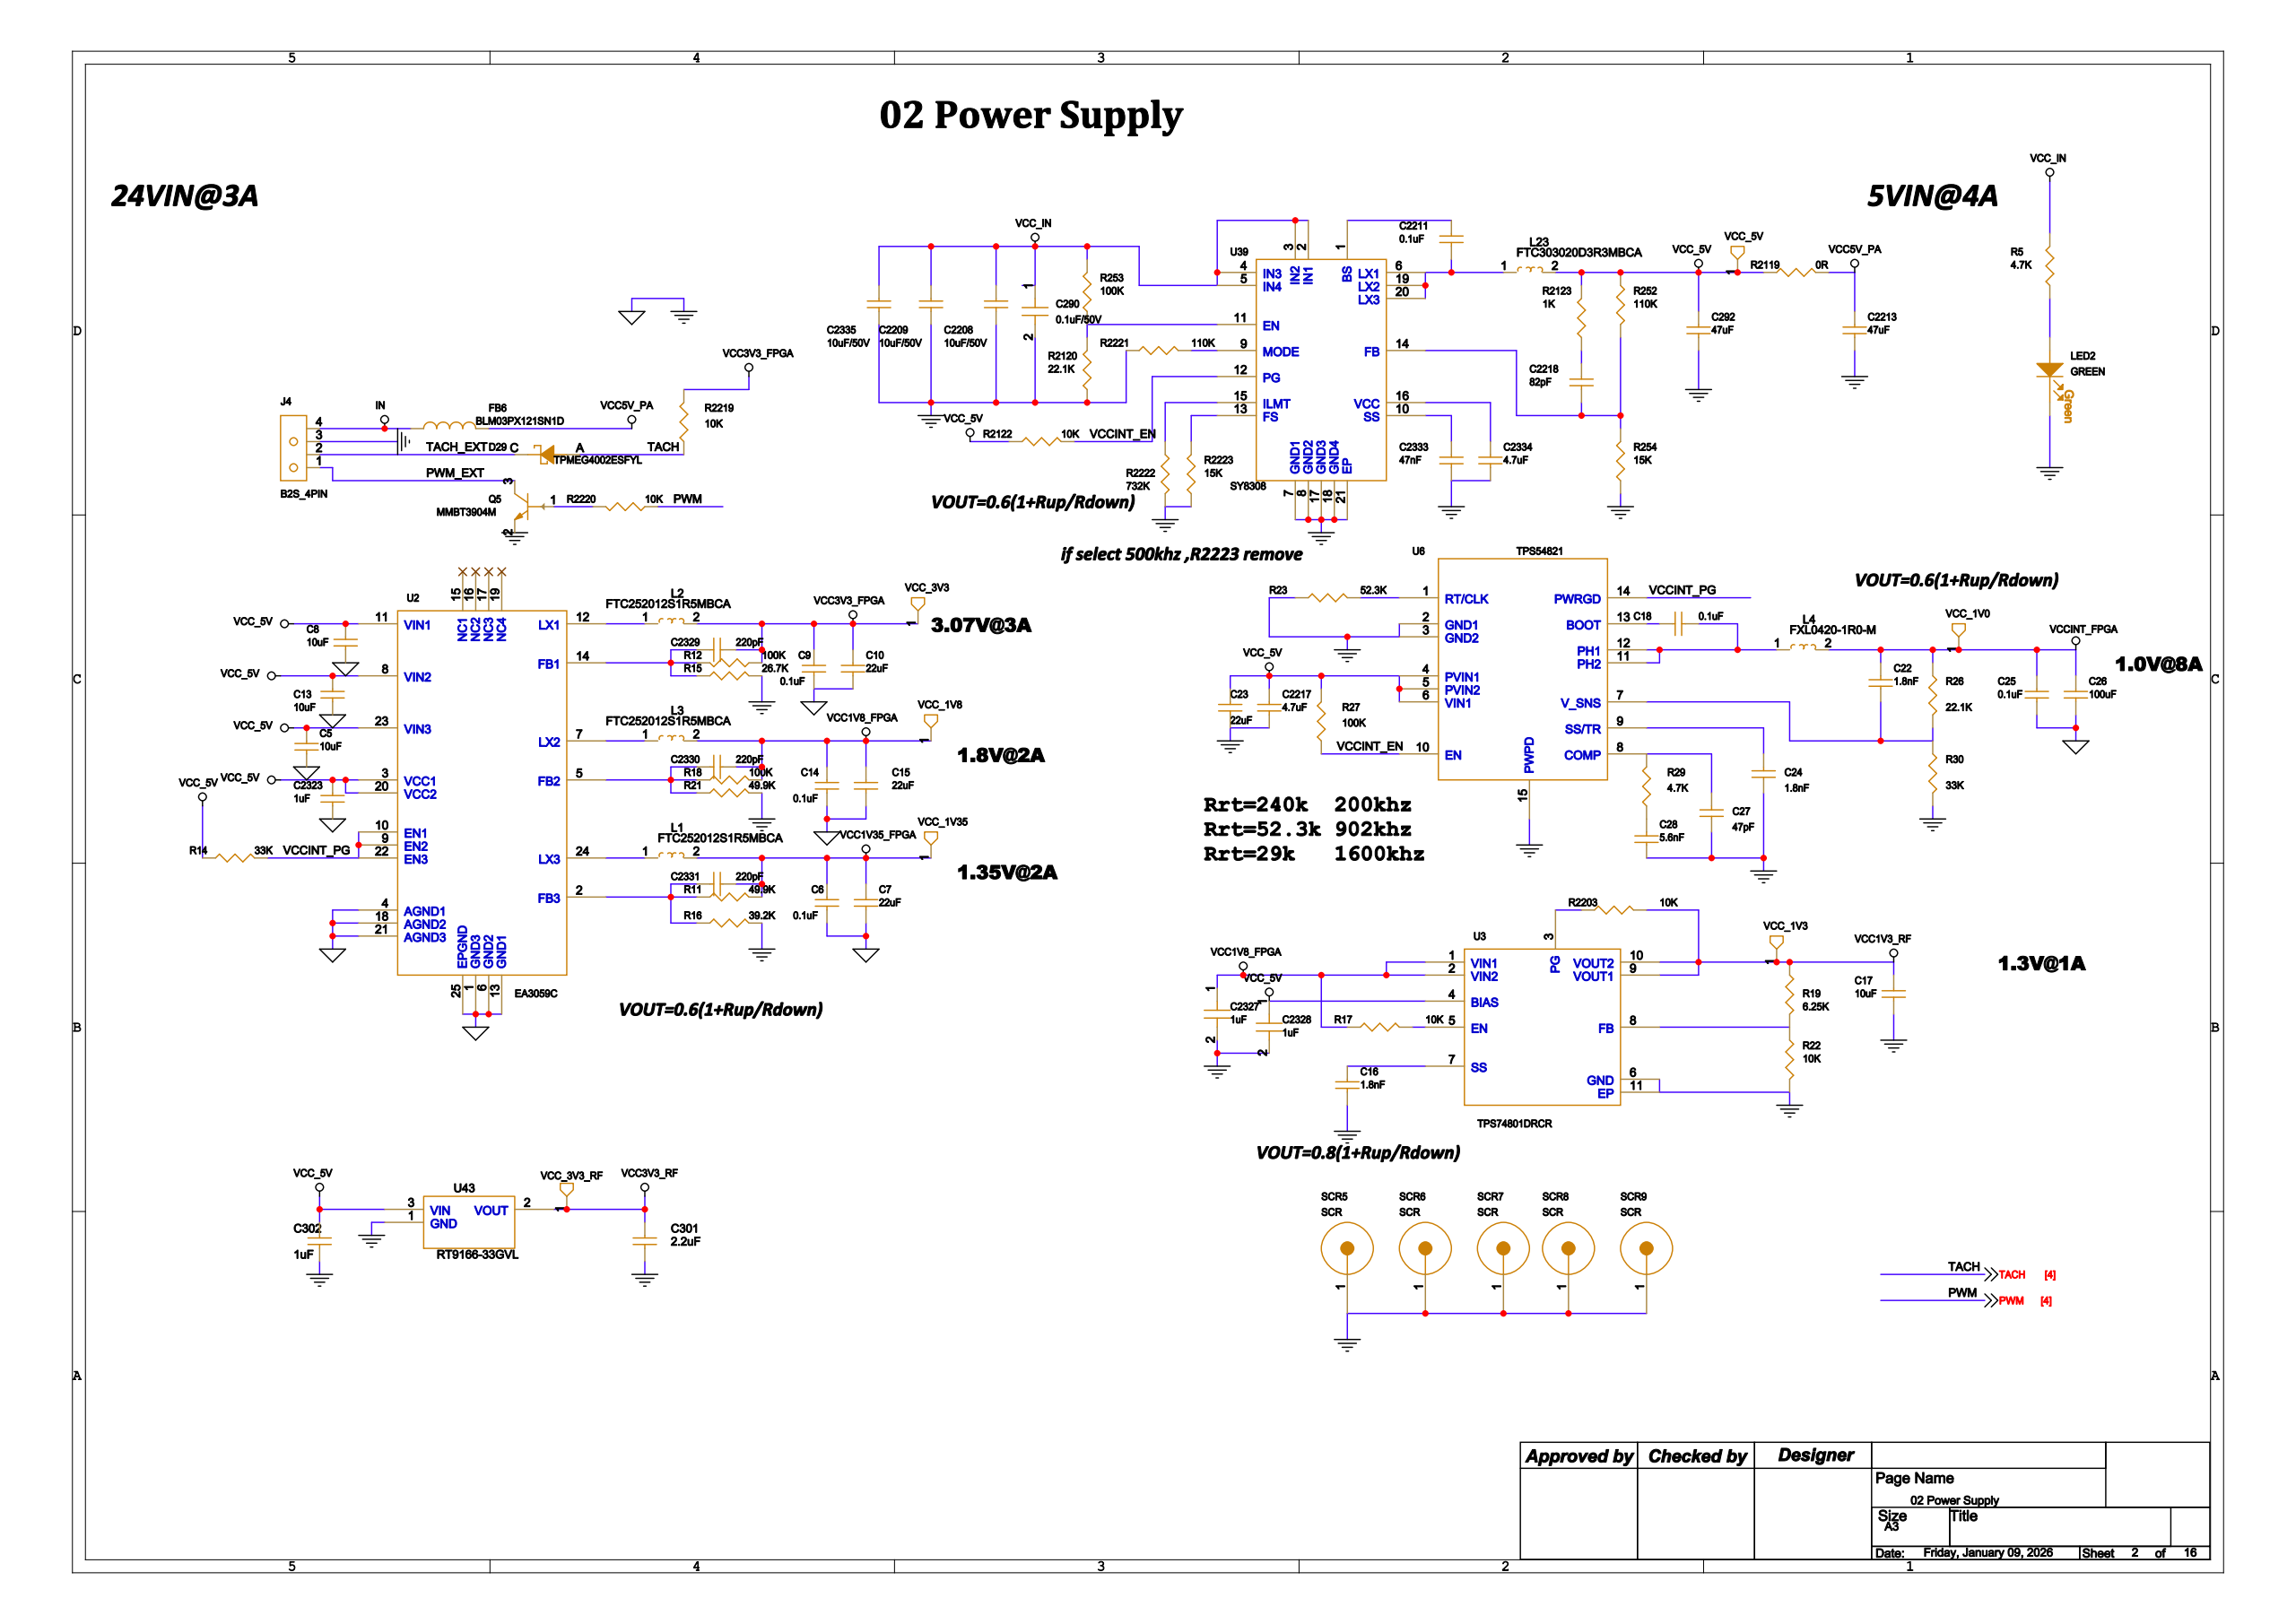Circuit board | Cadence Allegro | 442 parts | 326 nets | one sheet of the schematic
Parts on this sheet (reference | value | footprint):
C5 | 10uF | C0603
C6 | 0.1uF | C0201
C7 | 22uF | C0805
C8 | 10uF | C0603
C9 | 0.1uF | C0201
C10 | 22uF | C0805
C13 | 10uF | C0603
C16 | 1.8nF | C0201
C17 | 10uF | C0603
C22 | 1.8nF | C0201
C23 | 22uF | C0805
C24 | 1.8nF | C0201
C25 | 0.1uF | C0201
C26 | 100uF | C1206
C27 | 47pF | C0201
C28 | 5.6nF | C0201
C290 | 0.1uF/50V | C0402_D
C292 | 47uF | C0805
C301 | 2.2uF | C0201
C302 | 1uF | C0201
C2208 | 10uF/50V | C0805
C2209 | 10uF/50V | C0805
C2211 | 0.1uF | C0201
C2213 | 47uF | C0805
C2217 | 4.7uF | C0402_D
C2218 | 82pF | C0201
C2323 | 1uF | C0201
C2327 | 1uF | C0201
C2328 | 1uF | C0201
C2329 | 220pF | C0201
C2330 | 220pF | C0201
C2331 | 220pF | C0201
C2333 | 47nF | C0201
C2334 | 4.7uF | C0402_D
C2335 | 10uF/50V | C0805
D29 | TPMEG4002ESFYL | D0201
FB6 | BLM03PX121SN1D | L0201
J4 | B2S_4PIN | DIP1X4_1_27
L1 | FTC252012S1R5MBCA | 1008
L2 | FTC252012S1R5MBCA | 1008
L3 | FTC252012S1R5MBCA | 1008
L4 | FXL0420-1R0-M | SMD_0420
L23 | FTC303020D3R3MBCA | SMD_30X30
LED2 | GREEN | D0402
Q5 | MMBT3904M | SOT-723
R5 | 4.7K | R0201
R11 | 49.9K | R0201
R12 | 100K | R0201
R14 | 33K | R0201
R15 | 26.7K | R0201
R16 | 39.2K | R0201
R17 | 10K | R0201
R18 | 100K | R0201
R19 | 6.25K | R0201
R21 | 49.9K | R0201
R22 | 10K | R0201
R23 | 52.3K | R0201
R26 | 22.1K | R0201
R27 | 100K | R0201
R29 | 4.7K | R0201
R30 | 33K | R0201
R252 | 110K | R0201
R253 | 100K | R0201
R254 | 15K | R0201
R2119 | 0R | R0805
R2120 | 22.1K | R0201
R2122 | 10K | R0201
R2123 | 1K | R0201
R2203 | 10K | R0201
R2219 | 10K | R0201
R2220 | 10K | R0201
R2221 | 110K | R0201
R2222 | 732K | R0201
R2223 | 15K | R0201
SCR5 | SCR | HOLE2_2_4
SCR6 | SCR | HOLE2_2_4
SCR7 | SCR | HOLE2_2_4
SCR8 | SCR | HOLE2_2_4
SCR9 | SCR | HOLE2_2_4
U2 | EA3059C | QFN_24
U3 | TPS74801DRCR | TPS74901DRCR
U6 | TPS54821 | PVQFN14
U39 | SY8308 | SY8308RBC
U43 | RT9166-33GVL | SOT-23
VCC_1V0 | T POINT F | STP40
VCC_1V3 | T POINT F | STP40
VCC_1V8 | T POINT F | STP40
VCC_1V35 | T POINT F | STP40
VCC_3V3 | T POINT F | STP40
VCC_3V3_RF | T POINT F | STP40
Nets of these parts (net: part-pin ...):
VCC_5V: C5-1 C8-1 C13-1 C23-1 C292-1 C302-1 C2217-1 C2323-1 C2328-1 L23-2 R14-2 R27-1 R252-2 R2119-2 R2122-2 R2123-2 U3-4 U6-4 U6-5 U6-6 U43-3 U2-3 U2-8 U2-11 U2-20 U2-23
GND: C5-2 C6-2 C7-2 C8-2 C9-2 C10-2 C13-2 C16-2 C17-2 C23-2 C24-1 C25-2 C26-2 C27-1 C28-1 C290-2 C292-2 C301-2 C302-2 C2208-2 C2209-2 C2213-2 C2217-2 C2323-2 C2327-2 C2328-2 C2333-2 C2334-2 C2335-2 J4-3 LED2-2 Q5-2 R15-1 R16-1 R21-1 R22-2 R23-2 R30-1 R254-2 R2120-2 R2221-2 R2222-1 R2223-2 SCR5-1 SCR6-1 SCR7-1 SCR8-1 SCR9-1 U3-6 U3-11 U6-2 U6-3 U6-15 U43-1 U2-1 U2-4 U2-6 U2-13 U2-18 U2-21 U2-25 U39-7 U39-8 U39-17 U39-18 U39-21
N50602023: Q5-1 R2220-1
PWM_EXT: J4-1 Q5-3
N50559926: C2211-1 U39-1
N49332033: R253-2 R2120-1 U39-11
N49332062: C2218-2 R252-1 R254-1 U39-14
N50570197: R2223-1 U39-13
N50568877: R2222-2 U39-15
VCC_IN: C290-1 C2208-1 C2209-1 C2335-1 R5-1 R253-1 U39-2 U39-3 U39-4 U39-5
N49850498: C2211-2 L23-1 U39-6 U39-19 U39-20
N49852291: R2221-1 U39-9
VCCINT_EN: R27-2 R2122-1 U6-10 U39-12
N50568588: C2333-1 U39-10
N50568593: C2334-1 U39-16
N50104205: C2218-1 R2123-1
VCC3V3_RF: C301-1 U43-2 VCC_3V3_RF-1
VCC5V_PA: C2213-1 FB6-2 R2119-1
VCC1V8_FPGA: C2327-1 C2330-1 L3-2 R17-2 R18-1 U3-1 U3-2 VCC_1V8-1
IN: FB6-1 J4-4
TACH_EXT: D29-C J4-2
N48932072: L4-1 U6-11 U6-12
VCCINT_FPGA: C22-2 C25-1 C26-1 L4-2 R26-2 VCC_1V0-1
N50303974: C2329-2 R12-1 R15-2 U2-14
N48929185: C2331-2 R11-2 R16-2 U2-2
VCC1V35_FPGA: C6-1 C7-1 C2331-1 L1-2 R11-1 VCC_1V35-1
TACH: D29-A R2219-2
VCC3V3_FPGA: C9-1 C10-1 C2329-1 L2-2 R12-2 R2219-1 VCC_3V3-1
N50304507: C2330-2 R18-2 R21-2 U2-5
VCC1V3_RF: C17-1 R19-1 R2203-1 U3-9 U3-10 VCC_1V3-1
N47968047: LED2-1 R5-2
N50366213: R19-2 R22-1 U3-8
N50366211: R17-1 U3-5
N50366081: R2203-2 U3-3
N50366233: C16-1 U3-7
N48932070: U6-13
N48932134: C22-1 R26-1 R30-2 U6-7
N48932150: C24-2 U6-9
N48932166: C27-2 R29-1 U6-8
N489321741: C28-2 R29-2
N48929171: L1-1 U2-24
N48927210: L2-1 U2-12
N50304485: L3-1 U2-7
VCCINT_PG: R14-1 U6-14 U2-9 U2-10 U2-22
PWM: R2220-2
N48932055: R23-1 U6-1